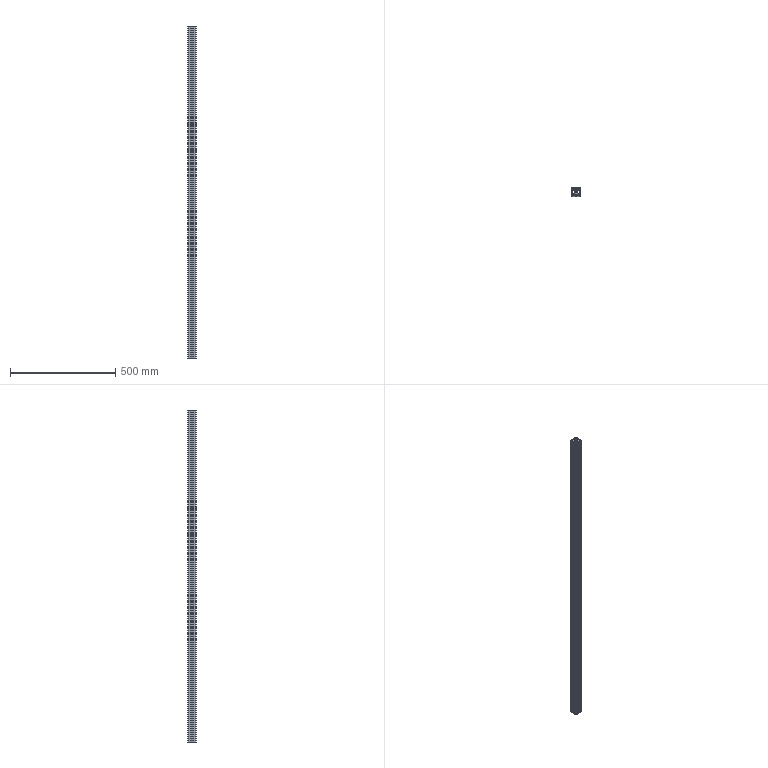Part | SolidWorks | features BaseBody 1, MoveFace 1 | 1 solid | 129 faces | box 40 x 40 x 1575 mm | volume 681555 mm3 | plane 102 | cylinder 27 | commonest cylinder face diameters 2 x8 1.5 x6 6.8 x5 6.6 x4 9 x4